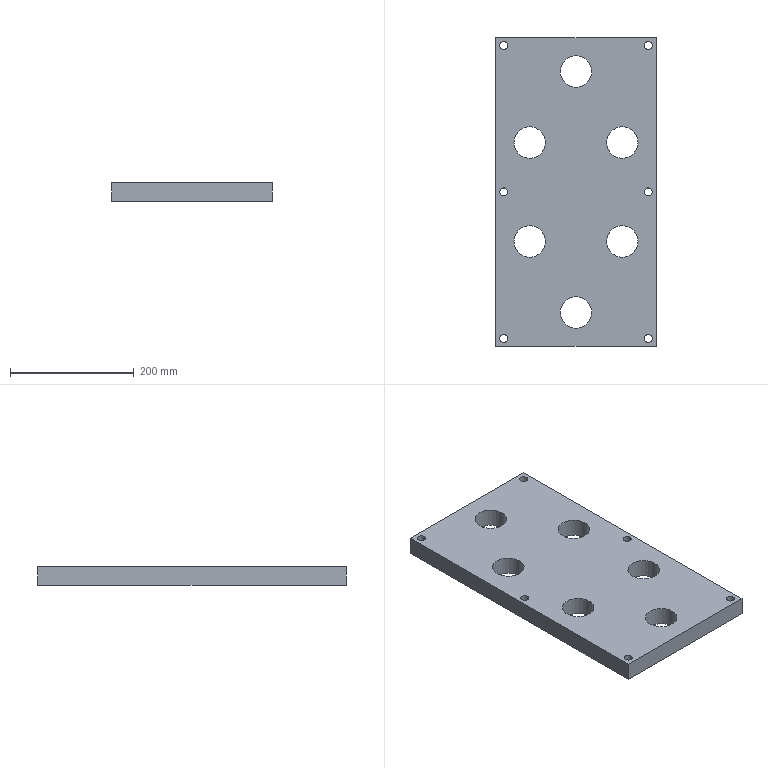Part | STEP file | SL2-MOLD_id738_xmt_txt | 1 solid | 30 faces | box 260 x 500 x 30 mm | volume 3495338 mm3 | cylinder 18 | plane 12 | commonest cylinder face diameters 13 x6 20 x6 51 x6
STEP:
#1=CARTESIAN_POINT('',(-49.5,170.,-244.));
#2=VERTEX_POINT('',#1);
#3=CARTESIAN_POINT('',(-75.,170.,-244.));
#4=DIRECTION('',(0.,0.,1.));
#5=DIRECTION('',(1.,0.,0.));
#6=AXIS2_PLACEMENT_3D('',#3,#4,#5);
#7=CIRCLE('',#6,25.5);
#8=EDGE_CURVE('',#2,#2,#7,.T.);
#9=ORIENTED_EDGE('',*,*,#8,.T.);
#10=EDGE_LOOP('',(#9));
#11=FACE_BOUND('',#10,.T.);
#12=CARTESIAN_POINT('',(-49.5,10.,-244.));
#13=VERTEX_POINT('',#12);
#14=CARTESIAN_POINT('',(-75.,10.,-244.));
#15=DIRECTION('',(0.,0.,1.));
#16=DIRECTION('',(1.,0.,0.));
#17=AXIS2_PLACEMENT_3D('',#14,#15,#16);
#18=CIRCLE('',#17,25.5);
#19=EDGE_CURVE('',#13,#13,#18,.T.);
#20=ORIENTED_EDGE('',*,*,#19,.T.);
#21=EDGE_LOOP('',(#20));
#22=FACE_BOUND('',#21,.T.);
#23=CARTESIAN_POINT('',(100.5,10.,-244.));
#24=VERTEX_POINT('',#23);
#25=CARTESIAN_POINT('',(75.,10.,-244.));
#26=DIRECTION('',(0.,0.,1.));
#27=DIRECTION('',(1.,0.,0.));
#28=AXIS2_PLACEMENT_3D('',#25,#26,#27);
#29=CIRCLE('',#28,25.5);
#30=EDGE_CURVE('',#24,#24,#29,.T.);
#31=ORIENTED_EDGE('',*,*,#30,.T.);
#32=EDGE_LOOP('',(#31));
#33=FACE_BOUND('',#32,.T.);
#34=CARTESIAN_POINT('',(127.,90.,-244.));
#35=VERTEX_POINT('',#34);
#36=CARTESIAN_POINT('',(117.,90.,-244.));
#37=DIRECTION('',(0.,0.,-1.));
#38=DIRECTION('',(1.,0.,0.));
#39=AXIS2_PLACEMENT_3D('',#36,#37,#38);
#40=CIRCLE('',#39,10.);
#41=EDGE_CURVE('',#35,#35,#40,.T.);
#42=ORIENTED_EDGE('',*,*,#41,.F.);
#43=EDGE_LOOP('',(#42));
#44=FACE_BOUND('',#43,.T.);
#45=CARTESIAN_POINT('',(127.,-147.,-244.));
#46=VERTEX_POINT('',#45);
#47=CARTESIAN_POINT('',(117.,-147.,-244.));
#48=DIRECTION('',(0.,0.,-1.));
#49=DIRECTION('',(1.,0.,0.));
#50=AXIS2_PLACEMENT_3D('',#47,#48,#49);
#51=CIRCLE('',#50,10.);
#52=EDGE_CURVE('',#46,#46,#51,.T.);
#53=ORIENTED_EDGE('',*,*,#52,.F.);
#54=EDGE_LOOP('',(#53));
#55=FACE_BOUND('',#54,.T.);
#56=CARTESIAN_POINT('',(-107.,-147.,-244.));
#57=VERTEX_POINT('',#56);
#58=CARTESIAN_POINT('',(-117.,-147.,-244.));
#59=DIRECTION('',(0.,0.,-1.));
#60=DIRECTION('',(1.,0.,0.));
#61=AXIS2_PLACEMENT_3D('',#58,#59,#60);
#62=CIRCLE('',#61,10.);
#63=EDGE_CURVE('',#57,#57,#62,.T.);
#64=ORIENTED_EDGE('',*,*,#63,.F.);
#65=EDGE_LOOP('',(#64));
#66=FACE_BOUND('',#65,.T.);
#67=CARTESIAN_POINT('',(-107.,90.,-244.));
#68=VERTEX_POINT('',#67);
#69=CARTESIAN_POINT('',(-117.,90.,-244.));
#70=DIRECTION('',(0.,0.,-1.));
#71=DIRECTION('',(1.,0.,0.));
#72=AXIS2_PLACEMENT_3D('',#69,#70,#71);
#73=CIRCLE('',#72,10.);
#74=EDGE_CURVE('',#68,#68,#73,.T.);
#75=ORIENTED_EDGE('',*,*,#74,.F.);
#76=EDGE_LOOP('',(#75));
#77=FACE_BOUND('',#76,.T.);
#78=CARTESIAN_POINT('',(-107.,327.,-244.));
#79=VERTEX_POINT('',#78);
#80=CARTESIAN_POINT('',(-117.,327.,-244.));
#81=DIRECTION('',(0.,0.,-1.));
#82=DIRECTION('',(1.,0.,0.));
#83=AXIS2_PLACEMENT_3D('',#80,#81,#82);
#84=CIRCLE('',#83,10.);
#85=EDGE_CURVE('',#79,#79,#84,.T.);
#86=ORIENTED_EDGE('',*,*,#85,.F.);
#87=EDGE_LOOP('',(#86));
#88=FACE_BOUND('',#87,.T.);
#89=CARTESIAN_POINT('',(127.,327.,-244.));
#90=VERTEX_POINT('',#89);
#91=CARTESIAN_POINT('',(117.,327.,-244.));
#92=DIRECTION('',(0.,0.,-1.));
#93=DIRECTION('',(1.,0.,0.));
#94=AXIS2_PLACEMENT_3D('',#91,#92,#93);
#95=CIRCLE('',#94,10.);
#96=EDGE_CURVE('',#90,#90,#95,.T.);
#97=ORIENTED_EDGE('',*,*,#96,.F.);
#98=EDGE_LOOP('',(#97));
#99=FACE_BOUND('',#98,.T.);
#100=CARTESIAN_POINT('',(-130.,340.,-244.));
#101=VERTEX_POINT('',#100);
#102=CARTESIAN_POINT('',(-130.,-160.,-244.));
#103=VERTEX_POINT('',#102);
#104=CARTESIAN_POINT('',(-130.,0.,-244.));
#105=DIRECTION('',(0.,-1.,0.));
#106=VECTOR('',#105,1.);
#107=LINE('',#104,#106);
#108=EDGE_CURVE('',#101,#103,#107,.T.);
#109=ORIENTED_EDGE('',*,*,#108,.F.);
#110=CARTESIAN_POINT('',(130.,340.,-244.));
#111=VERTEX_POINT('',#110);
#112=CARTESIAN_POINT('',(0.,340.,-244.));
#113=DIRECTION('',(-1.,0.,0.));
#114=VECTOR('',#113,1.);
#115=LINE('',#112,#114);
#116=EDGE_CURVE('',#111,#101,#115,.T.);
#117=ORIENTED_EDGE('',*,*,#116,.F.);
#118=CARTESIAN_POINT('',(130.,-160.,-244.));
#119=VERTEX_POINT('',#118);
#120=CARTESIAN_POINT('',(130.,0.,-244.));
#121=DIRECTION('',(0.,1.,0.));
#122=VECTOR('',#121,1.);
#123=LINE('',#120,#122);
#124=EDGE_CURVE('',#119,#111,#123,.T.);
#125=ORIENTED_EDGE('',*,*,#124,.F.);
#126=CARTESIAN_POINT('',(0.,-160.,-244.));
#127=DIRECTION('',(1.,0.,0.));
#128=VECTOR('',#127,1.);
#129=LINE('',#126,#128);
#130=EDGE_CURVE('',#103,#119,#129,.T.);
#131=ORIENTED_EDGE('',*,*,#130,.F.);
#132=EDGE_LOOP('',(#109,#117,#125,#131));
#133=FACE_BOUND('',#132,.T.);
#134=CARTESIAN_POINT('',(25.5,-105.,-244.));
#135=VERTEX_POINT('',#134);
#136=CARTESIAN_POINT('',(0.,-105.,-244.));
#137=DIRECTION('',(0.,0.,1.));
#138=DIRECTION('',(1.,0.,0.));
#139=AXIS2_PLACEMENT_3D('',#136,#137,#138);
#140=CIRCLE('',#139,25.5);
#141=EDGE_CURVE('',#135,#135,#140,.T.);
#142=ORIENTED_EDGE('',*,*,#141,.T.);
#143=EDGE_LOOP('',(#142));
#144=FACE_BOUND('',#143,.T.);
#145=CARTESIAN_POINT('',(100.5,170.,-244.));
#146=VERTEX_POINT('',#145);
#147=CARTESIAN_POINT('',(75.,170.,-244.));
#148=DIRECTION('',(0.,0.,1.));
#149=DIRECTION('',(1.,0.,0.));
#150=AXIS2_PLACEMENT_3D('',#147,#148,#149);
#151=CIRCLE('',#150,25.5);
#152=EDGE_CURVE('',#146,#146,#151,.T.);
#153=ORIENTED_EDGE('',*,*,#152,.T.);
#154=EDGE_LOOP('',(#153));
#155=FACE_BOUND('',#154,.T.);
#156=CARTESIAN_POINT('',(25.5,285.,-244.));
#157=VERTEX_POINT('',#156);
#158=CARTESIAN_POINT('',(0.,285.,-244.));
#159=DIRECTION('',(0.,0.,1.));
#160=DIRECTION('',(1.,0.,0.));
#161=AXIS2_PLACEMENT_3D('',#158,#159,#160);
#162=CIRCLE('',#161,25.5);
#163=EDGE_CURVE('',#157,#157,#162,.T.);
#164=ORIENTED_EDGE('',*,*,#163,.T.);
#165=EDGE_LOOP('',(#164));
#166=FACE_BOUND('',#165,.T.);
#167=CARTESIAN_POINT('',(0.,0.,-244.));
#168=DIRECTION('',(0.,0.,1.));
#169=DIRECTION('',(1.,0.,0.));
#170=AXIS2_PLACEMENT_3D('',#167,#168,#169);
#171=PLANE('',#170);
#172=ADVANCED_FACE('',(#11,#22,#33,#44,#55,#66,#77,#88,#99,#133,#144,#155,#166),#171,.F.);
#173=CARTESIAN_POINT('',(-130.,340.,-214.));
#174=VERTEX_POINT('',#173);
#175=CARTESIAN_POINT('',(-130.,-160.,-214.));
#176=VERTEX_POINT('',#175);
#177=CARTESIAN_POINT('',(-130.,90.,-214.));
#178=DIRECTION('',(0.,-1.,0.));
#179=VECTOR('',#178,1.);
#180=LINE('',#177,#179);
#181=EDGE_CURVE('',#174,#176,#180,.T.);
#182=ORIENTED_EDGE('',*,*,#181,.F.);
#183=CARTESIAN_POINT('',(-130.,340.,-244.));
#184=DIRECTION('',(0.,0.,1.));
#185=VECTOR('',#184,1.);
#186=LINE('',#183,#185);
#187=EDGE_CURVE('',#101,#174,#186,.T.);
#188=ORIENTED_EDGE('',*,*,#187,.F.);
#189=ORIENTED_EDGE('',*,*,#108,.T.);
#190=CARTESIAN_POINT('',(-130.,-160.,-244.));
#191=DIRECTION('',(0.,0.,-1.));
#192=VECTOR('',#191,1.);
#193=LINE('',#190,#192);
#194=EDGE_CURVE('',#176,#103,#193,.T.);
#195=ORIENTED_EDGE('',*,*,#194,.F.);
#196=EDGE_LOOP('',(#182,#188,#189,#195));
#197=FACE_OUTER_BOUND('',#196,.T.);
#198=CARTESIAN_POINT('',(-130.,90.,-179.));
#199=DIRECTION('',(-1.,0.,0.));
#200=DIRECTION('',(0.,0.,1.));
#201=AXIS2_PLACEMENT_3D('',#198,#199,#200);
#202=PLANE('',#201);
#203=ADVANCED_FACE('',(#197),#202,.T.);
#204=CARTESIAN_POINT('',(130.,340.,-214.));
#205=VERTEX_POINT('',#204);
#206=CARTESIAN_POINT('',(130.,-160.,-214.));
#207=VERTEX_POINT('',#206);
#208=CARTESIAN_POINT('',(130.,90.,-214.));
#209=DIRECTION('',(0.,-1.,0.));
#210=VECTOR('',#209,1.);
#211=LINE('',#208,#210);
#212=EDGE_CURVE('',#205,#207,#211,.T.);
#213=ORIENTED_EDGE('',*,*,#212,.T.);
#214=CARTESIAN_POINT('',(130.,-160.,-179.));
#215=DIRECTION('',(0.,0.,-1.));
#216=VECTOR('',#215,1.);
#217=LINE('',#214,#216);
#218=EDGE_CURVE('',#207,#119,#217,.T.);
#219=ORIENTED_EDGE('',*,*,#218,.T.);
#220=ORIENTED_EDGE('',*,*,#124,.T.);
#221=CARTESIAN_POINT('',(130.,340.,-244.));
#222=DIRECTION('',(0.,0.,-1.));
#223=VECTOR('',#222,1.);
#224=LINE('',#221,#223);
#225=EDGE_CURVE('',#205,#111,#224,.T.);
#226=ORIENTED_EDGE('',*,*,#225,.F.);
#227=EDGE_LOOP('',(#213,#219,#220,#226));
#228=FACE_OUTER_BOUND('',#227,.T.);
#229=CARTESIAN_POINT('',(130.,90.,-179.));
#230=DIRECTION('',(1.,0.,0.));
#231=DIRECTION('',(0.,0.,-1.));
#232=AXIS2_PLACEMENT_3D('',#229,#230,#231);
#233=PLANE('',#232);
#234=ADVANCED_FACE('',(#228),#233,.T.);
#235=CARTESIAN_POINT('',(0.,-160.,-214.));
#236=DIRECTION('',(-1.,0.,0.));
#237=VECTOR('',#236,1.);
#238=LINE('',#235,#237);
#239=EDGE_CURVE('',#207,#176,#238,.T.);
#240=ORIENTED_EDGE('',*,*,#239,.T.);
#241=ORIENTED_EDGE('',*,*,#194,.T.);
#242=ORIENTED_EDGE('',*,*,#130,.T.);
#243=ORIENTED_EDGE('',*,*,#218,.F.);
#244=EDGE_LOOP('',(#240,#241,#242,#243));
#245=FACE_OUTER_BOUND('',#244,.T.);
#246=CARTESIAN_POINT('',(0.,-160.,-244.));
#247=DIRECTION('',(0.,-1.,0.));
#248=DIRECTION('',(0.,0.,-1.));
#249=AXIS2_PLACEMENT_3D('',#246,#247,#248);
#250=PLANE('',#249);
#251=ADVANCED_FACE('',(#245),#250,.T.);
#252=CARTESIAN_POINT('',(0.,340.,-214.));
#253=DIRECTION('',(1.,0.,0.));
#254=VECTOR('',#253,1.);
#255=LINE('',#252,#254);
#256=EDGE_CURVE('',#174,#205,#255,.T.);
#257=ORIENTED_EDGE('',*,*,#256,.T.);
#258=ORIENTED_EDGE('',*,*,#225,.T.);
#259=ORIENTED_EDGE('',*,*,#116,.T.);
#260=ORIENTED_EDGE('',*,*,#187,.T.);
#261=EDGE_LOOP('',(#257,#258,#259,#260));
#262=FACE_OUTER_BOUND('',#261,.T.);
#263=CARTESIAN_POINT('',(0.,340.,-244.));
#264=DIRECTION('',(0.,1.,0.));
#265=DIRECTION('',(0.,0.,1.));
#266=AXIS2_PLACEMENT_3D('',#263,#264,#265);
#267=PLANE('',#266);
#268=ADVANCED_FACE('',(#262),#267,.T.);
#269=CARTESIAN_POINT('',(-100.5,170.,-214.));
#270=VERTEX_POINT('',#269);
#271=CARTESIAN_POINT('',(-75.,170.,-214.));
#272=DIRECTION('',(0.,0.,-1.));
#273=DIRECTION('',(-1.,0.,0.));
#274=AXIS2_PLACEMENT_3D('',#271,#272,#273);
#275=CIRCLE('',#274,25.5);
#276=EDGE_CURVE('',#270,#270,#275,.T.);
#277=ORIENTED_EDGE('',*,*,#276,.T.);
#278=EDGE_LOOP('',(#277));
#279=FACE_BOUND('',#278,.T.);
#280=CARTESIAN_POINT('',(-100.5,10.,-214.));
#281=VERTEX_POINT('',#280);
#282=CARTESIAN_POINT('',(-75.,10.,-214.));
#283=DIRECTION('',(0.,0.,-1.));
#284=DIRECTION('',(-1.,0.,0.));
#285=AXIS2_PLACEMENT_3D('',#282,#283,#284);
#286=CIRCLE('',#285,25.5);
#287=EDGE_CURVE('',#281,#281,#286,.T.);
#288=ORIENTED_EDGE('',*,*,#287,.T.);
#289=EDGE_LOOP('',(#288));
#290=FACE_BOUND('',#289,.T.);
#291=CARTESIAN_POINT('',(49.5,10.,-214.));
#292=VERTEX_POINT('',#291);
#293=CARTESIAN_POINT('',(75.,10.,-214.));
#294=DIRECTION('',(0.,0.,-1.));
#295=DIRECTION('',(-1.,0.,0.));
#296=AXIS2_PLACEMENT_3D('',#293,#294,#295);
#297=CIRCLE('',#296,25.5);
#298=EDGE_CURVE('',#292,#292,#297,.T.);
#299=ORIENTED_EDGE('',*,*,#298,.T.);
#300=EDGE_LOOP('',(#299));
#301=FACE_BOUND('',#300,.T.);
#302=CARTESIAN_POINT('',(-25.5,-105.,-214.));
#303=VERTEX_POINT('',#302);
#304=CARTESIAN_POINT('',(0.,-105.,-214.));
#305=DIRECTION('',(0.,0.,-1.));
#306=DIRECTION('',(-1.,0.,0.));
#307=AXIS2_PLACEMENT_3D('',#304,#305,#306);
#308=CIRCLE('',#307,25.5);
#309=EDGE_CURVE('',#303,#303,#308,.T.);
#310=ORIENTED_EDGE('',*,*,#309,.T.);
#311=EDGE_LOOP('',(#310));
#312=FACE_BOUND('',#311,.T.);
#313=CARTESIAN_POINT('',(-25.5,285.,-214.));
#314=VERTEX_POINT('',#313);
#315=CARTESIAN_POINT('',(0.,285.,-214.));
#316=DIRECTION('',(0.,0.,-1.));
#317=DIRECTION('',(-1.,0.,0.));
#318=AXIS2_PLACEMENT_3D('',#315,#316,#317);
#319=CIRCLE('',#318,25.5);
#320=EDGE_CURVE('',#314,#314,#319,.T.);
#321=ORIENTED_EDGE('',*,*,#320,.T.);
#322=EDGE_LOOP('',(#321));
#323=FACE_BOUND('',#322,.T.);
#324=CARTESIAN_POINT('',(49.5,170.,-214.));
#325=VERTEX_POINT('',#324);
#326=CARTESIAN_POINT('',(75.,170.,-214.));
#327=DIRECTION('',(0.,0.,-1.));
#328=DIRECTION('',(-1.,0.,0.));
#329=AXIS2_PLACEMENT_3D('',#326,#327,#328);
#330=CIRCLE('',#329,25.5);
#331=EDGE_CURVE('',#325,#325,#330,.T.);
#332=ORIENTED_EDGE('',*,*,#331,.T.);
#333=EDGE_LOOP('',(#332));
#334=FACE_BOUND('',#333,.T.);
#335=CARTESIAN_POINT('',(-123.5,-147.,-214.));
#336=VERTEX_POINT('',#335);
#337=CARTESIAN_POINT('',(-117.,-147.,-214.));
#338=DIRECTION('',(0.,0.,-1.));
#339=DIRECTION('',(-1.,0.,0.));
#340=AXIS2_PLACEMENT_3D('',#337,#338,#339);
#341=CIRCLE('',#340,6.5);
#342=EDGE_CURVE('',#336,#336,#341,.T.);
#343=ORIENTED_EDGE('',*,*,#342,.T.);
#344=EDGE_LOOP('',(#343));
#345=FACE_BOUND('',#344,.T.);
#346=CARTESIAN_POINT('',(110.5,-147.,-214.));
#347=VERTEX_POINT('',#346);
#348=CARTESIAN_POINT('',(117.,-147.,-214.));
#349=DIRECTION('',(0.,0.,-1.));
#350=DIRECTION('',(-1.,0.,0.));
#351=AXIS2_PLACEMENT_3D('',#348,#349,#350);
#352=CIRCLE('',#351,6.5);
#353=EDGE_CURVE('',#347,#347,#352,.T.);
#354=ORIENTED_EDGE('',*,*,#353,.T.);
#355=EDGE_LOOP('',(#354));
#356=FACE_BOUND('',#355,.T.);
#357=CARTESIAN_POINT('',(110.5,90.,-214.));
#358=VERTEX_POINT('',#357);
#359=CARTESIAN_POINT('',(117.,90.,-214.));
#360=DIRECTION('',(0.,0.,-1.));
#361=DIRECTION('',(-1.,0.,0.));
#362=AXIS2_PLACEMENT_3D('',#359,#360,#361);
#363=CIRCLE('',#362,6.5);
#364=EDGE_CURVE('',#358,#358,#363,.T.);
#365=ORIENTED_EDGE('',*,*,#364,.T.);
#366=EDGE_LOOP('',(#365));
#367=FACE_BOUND('',#366,.T.);
#368=CARTESIAN_POINT('',(-123.5,90.,-214.));
#369=VERTEX_POINT('',#368);
#370=CARTESIAN_POINT('',(-117.,90.,-214.));
#371=DIRECTION('',(0.,0.,-1.));
#372=DIRECTION('',(-1.,0.,0.));
#373=AXIS2_PLACEMENT_3D('',#370,#371,#372);
#374=CIRCLE('',#373,6.5);
#375=EDGE_CURVE('',#369,#369,#374,.T.);
#376=ORIENTED_EDGE('',*,*,#375,.T.);
#377=EDGE_LOOP('',(#376));
#378=FACE_BOUND('',#377,.T.);
#379=CARTESIAN_POINT('',(-123.5,327.,-214.));
#380=VERTEX_POINT('',#379);
#381=CARTESIAN_POINT('',(-117.,327.,-214.));
#382=DIRECTION('',(0.,0.,-1.));
#383=DIRECTION('',(-1.,0.,0.));
#384=AXIS2_PLACEMENT_3D('',#381,#382,#383);
#385=CIRCLE('',#384,6.5);
#386=EDGE_CURVE('',#380,#380,#385,.T.);
#387=ORIENTED_EDGE('',*,*,#386,.T.);
#388=EDGE_LOOP('',(#387));
#389=FACE_BOUND('',#388,.T.);
#390=CARTESIAN_POINT('',(110.5,327.,-214.));
#391=VERTEX_POINT('',#390);
#392=CARTESIAN_POINT('',(117.,327.,-214.));
#393=DIRECTION('',(0.,0.,-1.));
#394=DIRECTION('',(-1.,0.,0.));
#395=AXIS2_PLACEMENT_3D('',#392,#393,#394);
#396=CIRCLE('',#395,6.5);
#397=EDGE_CURVE('',#391,#391,#396,.T.);
#398=ORIENTED_EDGE('',*,*,#397,.T.);
#399=EDGE_LOOP('',(#398));
#400=FACE_BOUND('',#399,.T.);
#401=ORIENTED_EDGE('',*,*,#239,.F.);
#402=ORIENTED_EDGE('',*,*,#212,.F.);
#403=ORIENTED_EDGE('',*,*,#256,.F.);
#404=ORIENTED_EDGE('',*,*,#181,.T.);
#405=EDGE_LOOP('',(#401,#402,#403,#404));
#406=FACE_BOUND('',#405,.T.);
#407=CARTESIAN_POINT('',(0.,90.,-214.));
#408=DIRECTION('',(0.,0.,-1.));
#409=DIRECTION('',(-1.,0.,0.));
#410=AXIS2_PLACEMENT_3D('',#407,#408,#409);
#411=PLANE('',#410);
#412=ADVANCED_FACE('',(#279,#290,#301,#312,#323,#334,#345,#356,#367,#378,#389,#400,#406),#411,.F.);
#413=CARTESIAN_POINT('',(107.,327.,-232.));
#414=VERTEX_POINT('',#413);
#415=CARTESIAN_POINT('',(117.,327.,-232.));
#416=DIRECTION('',(0.,0.,1.));
#417=DIRECTION('',(-1.,0.,0.));
#418=AXIS2_PLACEMENT_3D('',#415,#416,#417);
#419=CIRCLE('',#418,10.);
#420=EDGE_CURVE('',#414,#414,#419,.T.);
#421=ORIENTED_EDGE('',*,*,#420,.T.);
#422=EDGE_LOOP('',(#421));
#423=FACE_BOUND('',#422,.T.);
#424=ORIENTED_EDGE('',*,*,#96,.T.);
#425=EDGE_LOOP('',(#424));
#426=FACE_BOUND('',#425,.T.);
#427=CARTESIAN_POINT('',(117.,327.,-267.));
#428=DIRECTION('',(0.,0.,1.));
#429=DIRECTION('',(1.,0.,0.));
#430=AXIS2_PLACEMENT_3D('',#427,#428,#429);
#431=CYLINDRICAL_SURFACE('',#430,10.);
#432=ADVANCED_FACE('',(#423,#426),#431,.F.);
#433=CARTESIAN_POINT('',(110.5,327.,-232.));
#434=VERTEX_POINT('',#433);
#435=CARTESIAN_POINT('',(117.,327.,-232.));
#436=DIRECTION('',(0.,0.,-1.));
#437=DIRECTION('',(-1.,0.,0.));
#438=AXIS2_PLACEMENT_3D('',#435,#436,#437);
#439=CIRCLE('',#438,6.5);
#440=EDGE_CURVE('',#434,#434,#439,.T.);
#441=ORIENTED_EDGE('',*,*,#440,.F.);
#442=EDGE_LOOP('',(#441));
#443=FACE_BOUND('',#442,.T.);
#444=ORIENTED_EDGE('',*,*,#420,.F.);
#445=EDGE_LOOP('',(#444));
#446=FACE_BOUND('',#445,.T.);
#447=CARTESIAN_POINT('',(117.,327.,-232.));
#448=DIRECTION('',(0.,0.,-1.));
#449=DIRECTION('',(-1.,0.,0.));
#450=AXIS2_PLACEMENT_3D('',#447,#448,#449);
#451=PLANE('',#450);
#452=ADVANCED_FACE('',(#443,#446),#451,.T.);
#453=CARTESIAN_POINT('',(-127.,327.,-232.));
#454=VERTEX_POINT('',#453);
#455=CARTESIAN_POINT('',(-117.,327.,-232.));
#456=DIRECTION('',(0.,0.,1.));
#457=DIRECTION('',(-1.,0.,0.));
#458=AXIS2_PLACEMENT_3D('',#455,#456,#457);
#459=CIRCLE('',#458,10.);
#460=EDGE_CURVE('',#454,#454,#459,.T.);
#461=ORIENTED_EDGE('',*,*,#460,.T.);
#462=EDGE_LOOP('',(#461));
#463=FACE_BOUND('',#462,.T.);
#464=ORIENTED_EDGE('',*,*,#85,.T.);
#465=EDGE_LOOP('',(#464));
#466=FACE_BOUND('',#465,.T.);
#467=CARTESIAN_POINT('',(-117.,327.,-267.));
#468=DIRECTION('',(0.,0.,1.));
#469=DIRECTION('',(1.,0.,0.));
#470=AXIS2_PLACEMENT_3D('',#467,#468,#469);
#471=CYLINDRICAL_SURFACE('',#470,10.);
#472=ADVANCED_FACE('',(#463,#466),#471,.F.);
#473=CARTESIAN_POINT('',(-123.5,327.,-232.));
#474=VERTEX_POINT('',#473);
#475=CARTESIAN_POINT('',(-117.,327.,-232.));
#476=DIRECTION('',(0.,0.,-1.));
#477=DIRECTION('',(-1.,0.,0.));
#478=AXIS2_PLACEMENT_3D('',#475,#476,#477);
#479=CIRCLE('',#478,6.5);
#480=EDGE_CURVE('',#474,#474,#479,.T.);
#481=ORIENTED_EDGE('',*,*,#480,.F.);
#482=EDGE_LOOP('',(#481));
#483=FACE_BOUND('',#482,.T.);
#484=ORIENTED_EDGE('',*,*,#460,.F.);
#485=EDGE_LOOP('',(#484));
#486=FACE_BOUND('',#485,.T.);
#487=CARTESIAN_POINT('',(-117.,327.,-232.));
#488=DIRECTION('',(0.,0.,-1.));
#489=DIRECTION('',(-1.,0.,0.));
#490=AXIS2_PLACEMENT_3D('',#487,#488,#489);
#491=PLANE('',#490);
#492=ADVANCED_FACE('',(#483,#486),#491,.T.);
#493=CARTESIAN_POINT('',(-127.,90.,-232.));
#494=VERTEX_POINT('',#493);
#495=CARTESIAN_POINT('',(-117.,90.,-232.));
#496=DIRECTION('',(0.,0.,1.));
#497=DIRECTION('',(-1.,0.,0.));
#498=AXIS2_PLACEMENT_3D('',#495,#496,#497);
#499=CIRCLE('',#498,10.);
#500=EDGE_CURVE('',#494,#494,#499,.T.);
#501=ORIENTED_EDGE('',*,*,#500,.T.);
#502=EDGE_LOOP('',(#501));
#503=FACE_BOUND('',#502,.T.);
#504=ORIENTED_EDGE('',*,*,#74,.T.);
#505=EDGE_LOOP('',(#504));
#506=FACE_BOUND('',#505,.T.);
#507=CARTESIAN_POINT('',(-117.,90.,-267.));
#508=DIRECTION('',(0.,0.,1.));
#509=DIRECTION('',(1.,0.,0.));
#510=AXIS2_PLACEMENT_3D('',#507,#508,#509);
#511=CYLINDRICAL_SURFACE('',#510,10.);
#512=ADVANCED_FACE('',(#503,#506),#511,.F.);
#513=CARTESIAN_POINT('',(-123.5,90.,-232.));
#514=VERTEX_POINT('',#513);
#515=CARTESIAN_POINT('',(-117.,90.,-232.));
#516=DIRECTION('',(0.,0.,-1.));
#517=DIRECTION('',(-1.,0.,0.));
#518=AXIS2_PLACEMENT_3D('',#515,#516,#517);
#519=CIRCLE('',#518,6.5);
#520=EDGE_CURVE('',#514,#514,#519,.T.);
#521=ORIENTED_EDGE('',*,*,#520,.F.);
#522=EDGE_LOOP('',(#521));
#523=FACE_BOUND('',#522,.T.);
#524=ORIENTED_EDGE('',*,*,#500,.F.);
#525=EDGE_LOOP('',(#524));
#526=FACE_BOUND('',#525,.T.);
#527=CARTESIAN_POINT('',(-117.,90.,-232.));
#528=DIRECTION('',(0.,0.,-1.));
#529=DIRECTION('',(-1.,0.,0.));
#530=AXIS2_PLACEMENT_3D('',#527,#528,#529);
#531=PLANE('',#530);
#532=ADVANCED_FACE('',(#523,#526),#531,.T.);
#533=CARTESIAN_POINT('',(-127.,-147.,-232.));
#534=VERTEX_POINT('',#533);
#535=CARTESIAN_POINT('',(-117.,-147.,-232.));
#536=DIRECTION('',(0.,0.,1.));
#537=DIRECTION('',(-1.,0.,0.));
#538=AXIS2_PLACEMENT_3D('',#535,#536,#537);
#539=CIRCLE('',#538,10.);
#540=EDGE_CURVE('',#534,#534,#539,.T.);
#541=ORIENTED_EDGE('',*,*,#540,.T.);
#542=EDGE_LOOP('',(#541));
#543=FACE_BOUND('',#542,.T.);
#544=ORIENTED_EDGE('',*,*,#63,.T.);
#545=EDGE_LOOP('',(#544));
#546=FACE_BOUND('',#545,.T.);
#547=CARTESIAN_POINT('',(-117.,-147.,-267.));
#548=DIRECTION('',(0.,0.,1.));
#549=DIRECTION('',(1.,0.,0.));
#550=AXIS2_PLACEMENT_3D('',#547,#548,#549);
#551=CYLINDRICAL_SURFACE('',#550,10.);
#552=ADVANCED_FACE('',(#543,#546),#551,.F.);
#553=CARTESIAN_POINT('',(-123.5,-147.,-232.));
#554=VERTEX_POINT('',#553);
#555=CARTESIAN_POINT('',(-117.,-147.,-232.));
#556=DIRECTION('',(0.,0.,-1.));
#557=DIRECTION('',(-1.,0.,0.));
#558=AXIS2_PLACEMENT_3D('',#555,#556,#557);
#559=CIRCLE('',#558,6.5);
#560=EDGE_CURVE('',#554,#554,#559,.T.);
#561=ORIENTED_EDGE('',*,*,#560,.F.);
#562=EDGE_LOOP('',(#561));
#563=FACE_BOUND('',#562,.T.);
#564=ORIENTED_EDGE('',*,*,#540,.F.);
#565=EDGE_LOOP('',(#564));
#566=FACE_BOUND('',#565,.T.);
#567=CARTESIAN_POINT('',(-117.,-147.,-232.));
#568=DIRECTION('',(0.,0.,-1.));
#569=DIRECTION('',(-1.,0.,0.));
#570=AXIS2_PLACEMENT_3D('',#567,#568,#569);
#571=PLANE('',#570);
#572=ADVANCED_FACE('',(#563,#566),#571,.T.);
#573=CARTESIAN_POINT('',(107.,-147.,-232.));
#574=VERTEX_POINT('',#573);
#575=CARTESIAN_POINT('',(117.,-147.,-232.));
#576=DIRECTION('',(0.,0.,1.));
#577=DIRECTION('',(-1.,0.,0.));
#578=AXIS2_PLACEMENT_3D('',#575,#576,#577);
#579=CIRCLE('',#578,10.);
#580=EDGE_CURVE('',#574,#574,#579,.T.);
#581=ORIENTED_EDGE('',*,*,#580,.T.);
#582=EDGE_LOOP('',(#581));
#583=FACE_BOUND('',#582,.T.);
#584=ORIENTED_EDGE('',*,*,#52,.T.);
#585=EDGE_LOOP('',(#584));
#586=FACE_BOUND('',#585,.T.);
#587=CARTESIAN_POINT('',(117.,-147.,-267.));
#588=DIRECTION('',(0.,0.,1.));
#589=DIRECTION('',(1.,0.,0.));
#590=AXIS2_PLACEMENT_3D('',#587,#588,#589);
#591=CYLINDRICAL_SURFACE('',#590,10.);
#592=ADVANCED_FACE('',(#583,#586),#591,.F.);
#593=CARTESIAN_POINT('',(110.5,-147.,-232.));
#594=VERTEX_POINT('',#593);
#595=CARTESIAN_POINT('',(117.,-147.,-232.));
#596=DIRECTION('',(0.,0.,-1.));
#597=DIRECTION('',(-1.,0.,0.));
#598=AXIS2_PLACEMENT_3D('',#595,#596,#597);
#599=CIRCLE('',#598,6.5);
#600=EDGE_CURVE('',#594,#594,#599,.T.);
#601=ORIENTED_EDGE('',*,*,#600,.F.);
#602=EDGE_LOOP('',(#601));
#603=FACE_BOUND('',#602,.T.);
#604=ORIENTED_EDGE('',*,*,#580,.F.);
#605=EDGE_LOOP('',(#604));
#606=FACE_BOUND('',#605,.T.);
#607=CARTESIAN_POINT('',(117.,-147.,-232.));
#608=DIRECTION('',(0.,0.,-1.));
#609=DIRECTION('',(-1.,0.,0.));
#610=AXIS2_PLACEMENT_3D('',#607,#608,#609);
#611=PLANE('',#610);
#612=ADVANCED_FACE('',(#603,#606),#611,.T.);
#613=CARTESIAN_POINT('',(107.,90.,-232.));
#614=VERTEX_POINT('',#613);
#615=CARTESIAN_POINT('',(117.,90.,-232.));
#616=DIRECTION('',(0.,0.,1.));
#617=DIRECTION('',(-1.,0.,0.));
#618=AXIS2_PLACEMENT_3D('',#615,#616,#617);
#619=CIRCLE('',#618,10.);
#620=EDGE_CURVE('',#614,#614,#619,.T.);
#621=ORIENTED_EDGE('',*,*,#620,.T.);
#622=EDGE_LOOP('',(#621));
#623=FACE_BOUND('',#622,.T.);
#624=ORIENTED_EDGE('',*,*,#41,.T.);
#625=EDGE_LOOP('',(#624));
#626=FACE_BOUND('',#625,.T.);
#627=CARTESIAN_POINT('',(117.,90.,-267.));
#628=DIRECTION('',(0.,0.,1.));
#629=DIRECTION('',(1.,0.,0.));
#630=AXIS2_PLACEMENT_3D('',#627,#628,#629);
#631=CYLINDRICAL_SURFACE('',#630,10.);
#632=ADVANCED_FACE('',(#623,#626),#631,.F.);
#633=CARTESIAN_POINT('',(110.5,90.,-232.));
#634=VERTEX_POINT('',#633);
#635=CARTESIAN_POINT('',(117.,90.,-232.));
#636=DIRECTION('',(0.,0.,-1.));
#637=DIRECTION('',(-1.,0.,0.));
#638=AXIS2_PLACEMENT_3D('',#635,#636,#637);
#639=CIRCLE('',#638,6.5);
#640=EDGE_CURVE('',#634,#634,#639,.T.);
#641=ORIENTED_EDGE('',*,*,#640,.F.);
#642=EDGE_LOOP('',(#641));
#643=FACE_BOUND('',#642,.T.);
#644=ORIENTED_EDGE('',*,*,#620,.F.);
#645=EDGE_LOOP('',(#644));
#646=FACE_BOUND('',#645,.T.);
#647=CARTESIAN_POINT('',(117.,90.,-232.));
#648=DIRECTION('',(0.,0.,-1.));
#649=DIRECTION('',(-1.,0.,0.));
#650=AXIS2_PLACEMENT_3D('',#647,#648,#649);
#651=PLANE('',#650);
#652=ADVANCED_FACE('',(#643,#646),#651,.T.);
#653=ORIENTED_EDGE('',*,*,#440,.T.);
#654=EDGE_LOOP('',(#653));
#655=FACE_BOUND('',#654,.T.);
#656=ORIENTED_EDGE('',*,*,#397,.F.);
#657=EDGE_LOOP('',(#656));
#658=FACE_BOUND('',#657,.T.);
#659=CARTESIAN_POINT('',(117.,327.,263.));
#660=DIRECTION('',(0.,0.,-1.));
#661=DIRECTION('',(-1.,0.,0.));
#662=AXIS2_PLACEMENT_3D('',#659,#660,#661);
#663=CYLINDRICAL_SURFACE('',#662,6.5);
#664=ADVANCED_FACE('',(#655,#658),#663,.F.);
#665=ORIENTED_EDGE('',*,*,#480,.T.);
#666=EDGE_LOOP('',(#665));
#667=FACE_BOUND('',#666,.T.);
#668=ORIENTED_EDGE('',*,*,#386,.F.);
#669=EDGE_LOOP('',(#668));
#670=FACE_BOUND('',#669,.T.);
#671=CARTESIAN_POINT('',(-117.,327.,263.));
#672=DIRECTION('',(0.,0.,-1.));
#673=DIRECTION('',(-1.,0.,0.));
#674=AXIS2_PLACEMENT_3D('',#671,#672,#673);
#675=CYLINDRICAL_SURFACE('',#674,6.5);
#676=ADVANCED_FACE('',(#667,#670),#675,.F.);
#677=ORIENTED_EDGE('',*,*,#520,.T.);
#678=EDGE_LOOP('',(#677));
#679=FACE_BOUND('',#678,.T.);
#680=ORIENTED_EDGE('',*,*,#375,.F.);
#681=EDGE_LOOP('',(#680));
#682=FACE_BOUND('',#681,.T.);
#683=CARTESIAN_POINT('',(-117.,90.,263.));
#684=DIRECTION('',(0.,0.,-1.));
#685=DIRECTION('',(-1.,0.,0.));
#686=AXIS2_PLACEMENT_3D('',#683,#684,#685);
#687=CYLINDRICAL_SURFACE('',#686,6.5);
#688=ADVANCED_FACE('',(#679,#682),#687,.F.);
#689=ORIENTED_EDGE('',*,*,#640,.T.);
#690=EDGE_LOOP('',(#689));
#691=FACE_BOUND('',#690,.T.);
#692=ORIENTED_EDGE('',*,*,#364,.F.);
#693=EDGE_LOOP('',(#692));
#694=FACE_BOUND('',#693,.T.);
#695=CARTESIAN_POINT('',(117.,90.,263.));
#696=DIRECTION('',(0.,0.,-1.));
#697=DIRECTION('',(-1.,0.,0.));
#698=AXIS2_PLACEMENT_3D('',#695,#696,#697);
#699=CYLINDRICAL_SURFACE('',#698,6.5);
#700=ADVANCED_FACE('',(#691,#694),#699,.F.);
#701=ORIENTED_EDGE('',*,*,#600,.T.);
#702=EDGE_LOOP('',(#701));
#703=FACE_BOUND('',#702,.T.);
#704=ORIENTED_EDGE('',*,*,#353,.F.);
#705=EDGE_LOOP('',(#704));
#706=FACE_BOUND('',#705,.T.);
#707=CARTESIAN_POINT('',(117.,-147.,263.));
#708=DIRECTION('',(0.,0.,-1.));
#709=DIRECTION('',(-1.,0.,0.));
#710=AXIS2_PLACEMENT_3D('',#707,#708,#709);
#711=CYLINDRICAL_SURFACE('',#710,6.5);
#712=ADVANCED_FACE('',(#703,#706),#711,.F.);
#713=ORIENTED_EDGE('',*,*,#560,.T.);
#714=EDGE_LOOP('',(#713));
#715=FACE_BOUND('',#714,.T.);
#716=ORIENTED_EDGE('',*,*,#342,.F.);
#717=EDGE_LOOP('',(#716));
#718=FACE_BOUND('',#717,.T.);
#719=CARTESIAN_POINT('',(-117.,-147.,263.));
#720=DIRECTION('',(0.,0.,-1.));
#721=DIRECTION('',(-1.,0.,0.));
#722=AXIS2_PLACEMENT_3D('',#719,#720,#721);
#723=CYLINDRICAL_SURFACE('',#722,6.5);
#724=ADVANCED_FACE('',(#715,#718),#723,.F.);
#725=ORIENTED_EDGE('',*,*,#331,.F.);
#726=EDGE_LOOP('',(#725));
#727=FACE_BOUND('',#726,.T.);
#728=ORIENTED_EDGE('',*,*,#152,.F.);
#729=EDGE_LOOP('',(#728));
#730=FACE_BOUND('',#729,.T.);
#731=CARTESIAN_POINT('',(75.,170.,-244.));
#732=DIRECTION('',(0.,0.,1.));
#733=DIRECTION('',(1.,0.,0.));
#734=AXIS2_PLACEMENT_3D('',#731,#732,#733);
#735=CYLINDRICAL_SURFACE('',#734,25.5);
#736=ADVANCED_FACE('',(#727,#730),#735,.F.);
#737=ORIENTED_EDGE('',*,*,#320,.F.);
#738=EDGE_LOOP('',(#737));
#739=FACE_BOUND('',#738,.T.);
#740=ORIENTED_EDGE('',*,*,#163,.F.);
#741=EDGE_LOOP('',(#740));
#742=FACE_BOUND('',#741,.T.);
#743=CARTESIAN_POINT('',(0.,285.,-244.));
#744=DIRECTION('',(0.,0.,1.));
#745=DIRECTION('',(1.,0.,0.));
#746=AXIS2_PLACEMENT_3D('',#743,#744,#745);
#747=CYLINDRICAL_SURFACE('',#746,25.5);
#748=ADVANCED_FACE('',(#739,#742),#747,.F.);
#749=ORIENTED_EDGE('',*,*,#309,.F.);
#750=EDGE_LOOP('',(#749));
#751=FACE_BOUND('',#750,.T.);
#752=ORIENTED_EDGE('',*,*,#141,.F.);
#753=EDGE_LOOP('',(#752));
#754=FACE_BOUND('',#753,.T.);
#755=CARTESIAN_POINT('',(0.,-105.,-244.));
#756=DIRECTION('',(0.,0.,1.));
#757=DIRECTION('',(-1.,0.,0.));
#758=AXIS2_PLACEMENT_3D('',#755,#756,#757);
#759=CYLINDRICAL_SURFACE('',#758,25.5);
#760=ADVANCED_FACE('',(#751,#754),#759,.F.);
#761=ORIENTED_EDGE('',*,*,#298,.F.);
#762=EDGE_LOOP('',(#761));
#763=FACE_BOUND('',#762,.T.);
#764=ORIENTED_EDGE('',*,*,#30,.F.);
#765=EDGE_LOOP('',(#764));
#766=FACE_BOUND('',#765,.T.);
#767=CARTESIAN_POINT('',(75.,10.,-244.));
#768=DIRECTION('',(0.,0.,1.));
#769=DIRECTION('',(-1.,0.,0.));
#770=AXIS2_PLACEMENT_3D('',#767,#768,#769);
#771=CYLINDRICAL_SURFACE('',#770,25.5);
#772=ADVANCED_FACE('',(#763,#766),#771,.F.);
#773=ORIENTED_EDGE('',*,*,#287,.F.);
#774=EDGE_LOOP('',(#773));
#775=FACE_BOUND('',#774,.T.);
#776=ORIENTED_EDGE('',*,*,#19,.F.);
#777=EDGE_LOOP('',(#776));
#778=FACE_BOUND('',#777,.T.);
#779=CARTESIAN_POINT('',(-75.,10.,-244.));
#780=DIRECTION('',(0.,0.,1.));
#781=DIRECTION('',(-1.,0.,0.));
#782=AXIS2_PLACEMENT_3D('',#779,#780,#781);
#783=CYLINDRICAL_SURFACE('',#782,25.5);
#784=ADVANCED_FACE('',(#775,#778),#783,.F.);
#785=ORIENTED_EDGE('',*,*,#276,.F.);
#786=EDGE_LOOP('',(#785));
#787=FACE_BOUND('',#786,.T.);
#788=ORIENTED_EDGE('',*,*,#8,.F.);
#789=EDGE_LOOP('',(#788));
#790=FACE_BOUND('',#789,.T.);
#791=CARTESIAN_POINT('',(-75.,170.,-244.));
#792=DIRECTION('',(0.,0.,1.));
#793=DIRECTION('',(1.,0.,0.));
#794=AXIS2_PLACEMENT_3D('',#791,#792,#793);
#795=CYLINDRICAL_SURFACE('',#794,25.5);
#796=ADVANCED_FACE('',(#787,#790),#795,.F.);
#797=CLOSED_SHELL('',(#172,#203,#234,#251,#268,#412,#432,#452,#472,#492,#512,#532,#552,#572,#592,#612,#632,#652,#664,#676,#688,#700,#712,#724,#736,#748,#760,#772,#784,#796));
#798=MANIFOLD_SOLID_BREP('',#797);
#799=(LENGTH_UNIT()NAMED_UNIT(*)SI_UNIT(.MILLI.,.METRE.));
#800=UNCERTAINTY_MEASURE_WITH_UNIT(LENGTH_MEASURE(0.00002),#799,'','');
#801=(NAMED_UNIT(*)PLANE_ANGLE_UNIT()SI_UNIT($,.RADIAN.));
#802=PLANE_ANGLE_MEASURE_WITH_UNIT(PLANE_ANGLE_MEASURE(0.01745),#801);
#803=DIMENSIONAL_EXPONENTS(0.,0.,0.,0.,0.,0.,0.);
#804=(CONVERSION_BASED_UNIT('DEGREE',#802)NAMED_UNIT(#803)PLANE_ANGLE_UNIT());
#805=(NAMED_UNIT(*)SI_UNIT($,.STERADIAN.)SOLID_ANGLE_UNIT());
#806=(GEOMETRIC_REPRESENTATION_CONTEXT(3)GLOBAL_UNCERTAINTY_ASSIGNED_CONTEXT((#800))GLOBAL_UNIT_ASSIGNED_CONTEXT((#799,#804,#805))REPRESENTATION_CONTEXT('',''));
#807=ADVANCED_BREP_SHAPE_REPRESENTATION('',(#798),#806);